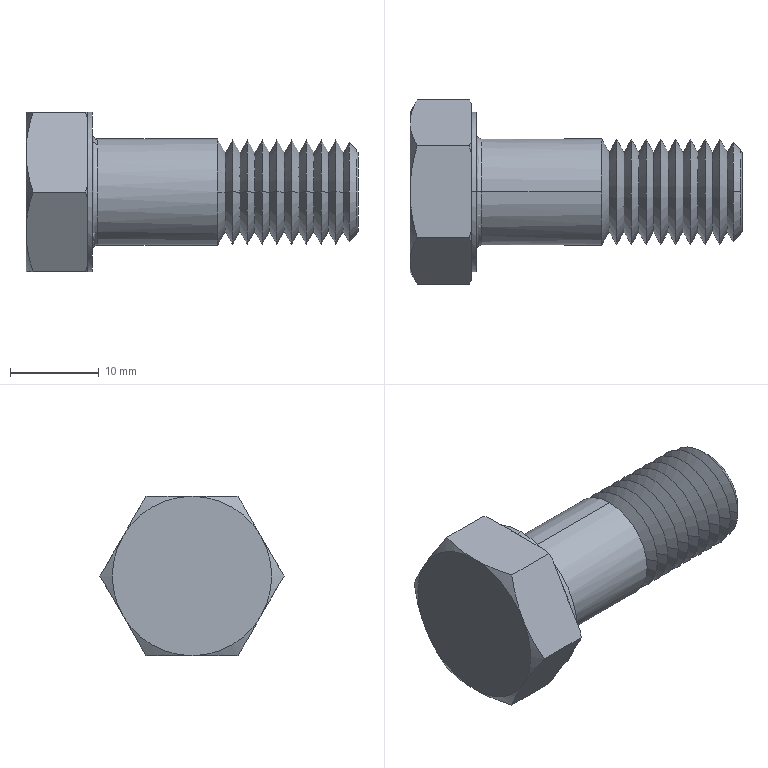Part | SolidWorks | features RevCut 4, Chamfer 1, Extrusion 1, Fillet 1, LPattern 1, Revolution 1 | 1 solid | 73 faces | box 37.5 x 20.785 x 18 mm | volume 5037 mm3 | cone 52 | plane 15 | cylinder 4 | torus 2 | commonest cylinder face diameters 12 x2 18 x2